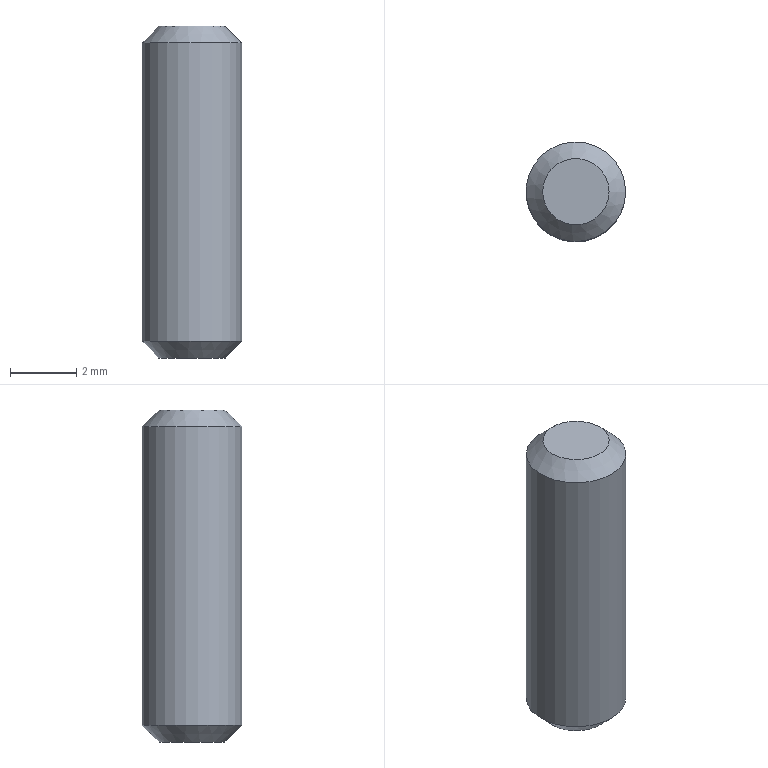Part | NX | 1 solid | 5 faces | box 3 x 3 x 10 mm | volume 68.591 mm3 | plane 2 | cone 2 | cylinder 1 | commonest cylinder face diameters 3 x1
STEP:
#1=CARTESIAN_POINT('',(1.5,0.,-4.5));
#2=VERTEX_POINT('',#1);
#3=CARTESIAN_POINT('',(0.,0.,-4.5));
#4=DIRECTION('',(0.,0.,1.));
#5=DIRECTION('',(1.,0.,0.));
#6=AXIS2_PLACEMENT_3D('',#3,#4,#5);
#7=CIRCLE('',#6,1.5);
#8=EDGE_CURVE('',#2,#2,#7,.T.);
#9=ORIENTED_EDGE('',*,*,#8,.T.);
#10=EDGE_LOOP('',(#9));
#11=FACE_BOUND('',#10,.T.);
#12=CARTESIAN_POINT('',(1.5,0.,4.5));
#13=VERTEX_POINT('',#12);
#14=CARTESIAN_POINT('',(0.,0.,4.5));
#15=DIRECTION('',(0.,0.,1.));
#16=DIRECTION('',(1.,0.,0.));
#17=AXIS2_PLACEMENT_3D('',#14,#15,#16);
#18=CIRCLE('',#17,1.5);
#19=EDGE_CURVE('',#13,#13,#18,.F.);
#20=ORIENTED_EDGE('',*,*,#19,.T.);
#21=EDGE_LOOP('',(#20));
#22=FACE_BOUND('',#21,.T.);
#23=CARTESIAN_POINT('',(0.,0.,5.));
#24=DIRECTION('',(0.,0.,-1.));
#25=DIRECTION('',(-1.,0.,0.));
#26=AXIS2_PLACEMENT_3D('',#23,#24,#25);
#27=CYLINDRICAL_SURFACE('',#26,1.5);
#28=ADVANCED_FACE('',(#11,#22),#27,.T.);
#29=CARTESIAN_POINT('',(1.,0.,5.));
#30=VERTEX_POINT('',#29);
#31=CARTESIAN_POINT('',(0.,0.,5.));
#32=DIRECTION('',(0.,0.,1.));
#33=DIRECTION('',(1.,0.,0.));
#34=AXIS2_PLACEMENT_3D('',#31,#32,#33);
#35=CIRCLE('',#34,1.);
#36=EDGE_CURVE('',#30,#30,#35,.T.);
#37=ORIENTED_EDGE('',*,*,#36,.T.);
#38=EDGE_LOOP('',(#37));
#39=FACE_BOUND('',#38,.T.);
#40=CARTESIAN_POINT('',(0.,0.,5.));
#41=DIRECTION('',(0.,0.,1.));
#42=DIRECTION('',(1.,0.,0.));
#43=AXIS2_PLACEMENT_3D('',#40,#41,#42);
#44=PLANE('',#43);
#45=ADVANCED_FACE('',(#39),#44,.T.);
#46=CARTESIAN_POINT('',(1.,0.,-5.));
#47=VERTEX_POINT('',#46);
#48=CARTESIAN_POINT('',(0.,0.,-5.));
#49=DIRECTION('',(0.,0.,1.));
#50=DIRECTION('',(1.,0.,0.));
#51=AXIS2_PLACEMENT_3D('',#48,#49,#50);
#52=CIRCLE('',#51,1.);
#53=EDGE_CURVE('',#47,#47,#52,.F.);
#54=ORIENTED_EDGE('',*,*,#53,.T.);
#55=EDGE_LOOP('',(#54));
#56=FACE_BOUND('',#55,.T.);
#57=CARTESIAN_POINT('',(0.,0.,-5.));
#58=DIRECTION('',(0.,0.,1.));
#59=DIRECTION('',(1.,0.,0.));
#60=AXIS2_PLACEMENT_3D('',#57,#58,#59);
#61=PLANE('',#60);
#62=ADVANCED_FACE('',(#56),#61,.F.);
#63=ORIENTED_EDGE('',*,*,#53,.F.);
#64=EDGE_LOOP('',(#63));
#65=FACE_BOUND('',#64,.T.);
#66=ORIENTED_EDGE('',*,*,#8,.F.);
#67=EDGE_LOOP('',(#66));
#68=FACE_BOUND('',#67,.T.);
#69=CARTESIAN_POINT('',(0.,0.,-4.5));
#70=DIRECTION('',(0.,0.,1.));
#71=DIRECTION('',(1.,0.,0.));
#72=AXIS2_PLACEMENT_3D('',#69,#70,#71);
#73=CONICAL_SURFACE('',#72,1.5,0.7854);
#74=ADVANCED_FACE('',(#65,#68),#73,.T.);
#75=ORIENTED_EDGE('',*,*,#19,.F.);
#76=EDGE_LOOP('',(#75));
#77=FACE_BOUND('',#76,.T.);
#78=ORIENTED_EDGE('',*,*,#36,.F.);
#79=EDGE_LOOP('',(#78));
#80=FACE_BOUND('',#79,.T.);
#81=CARTESIAN_POINT('',(0.,0.,5.));
#82=DIRECTION('',(0.,0.,-1.));
#83=DIRECTION('',(-1.,0.,0.));
#84=AXIS2_PLACEMENT_3D('',#81,#82,#83);
#85=CONICAL_SURFACE('',#84,1.,0.7854);
#86=ADVANCED_FACE('',(#77,#80),#85,.T.);
#87=CLOSED_SHELL('',(#28,#45,#62,#74,#86));
#88=MANIFOLD_SOLID_BREP('',#87);
#89=(LENGTH_UNIT()NAMED_UNIT(*)SI_UNIT(.MILLI.,.METRE.));
#90=UNCERTAINTY_MEASURE_WITH_UNIT(LENGTH_MEASURE(0.00001),#89,'','');
#91=(NAMED_UNIT(*)PLANE_ANGLE_UNIT()SI_UNIT($,.RADIAN.));
#92=(NAMED_UNIT(*)SI_UNIT($,.STERADIAN.)SOLID_ANGLE_UNIT());
#93=(GEOMETRIC_REPRESENTATION_CONTEXT(3)GLOBAL_UNCERTAINTY_ASSIGNED_CONTEXT((#90))GLOBAL_UNIT_ASSIGNED_CONTEXT((#89,#91,#92))REPRESENTATION_CONTEXT('',''));
#94=ADVANCED_BREP_SHAPE_REPRESENTATION('',(#88),#93);